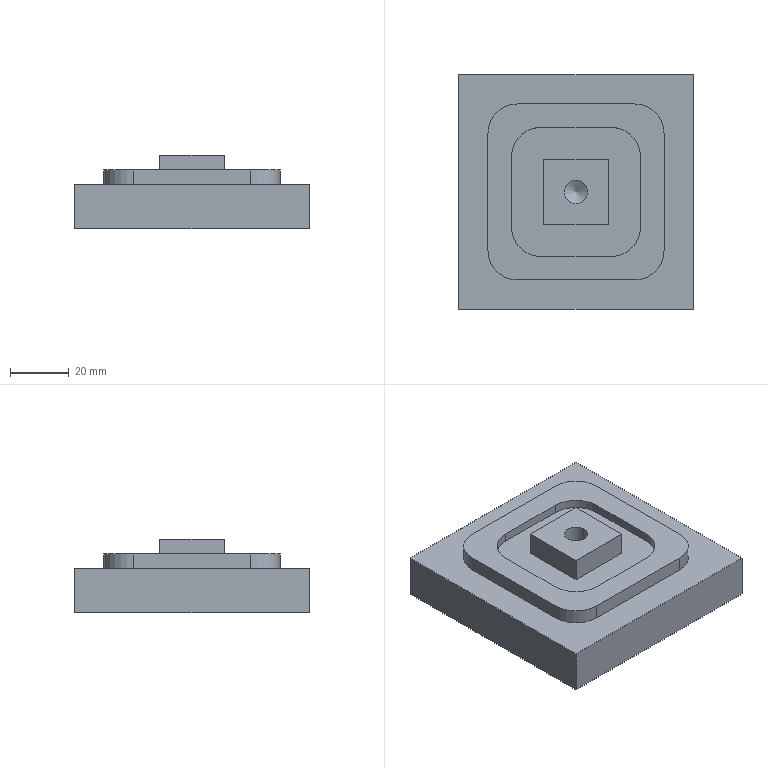Part | NX | 1 solid | 31 faces | box 80 x 80 x 25 mm | volume 111450 mm3 | plane 21 | cylinder 9 | cone 1 | commonest cylinder face diameters 20 x8 8 x1
STEP:
#1=CARTESIAN_POINT('',(-12.,-22.,17.));
#2=VERTEX_POINT('',#1);
#3=CARTESIAN_POINT('',(12.,-22.,17.));
#4=VERTEX_POINT('',#3);
#5=CARTESIAN_POINT('',(-22.,-22.,17.));
#6=DIRECTION('',(1.,0.,0.));
#7=VECTOR('',#6,1000.);
#8=LINE('',#5,#7);
#9=EDGE_CURVE('',#2,#4,#8,.T.);
#10=ORIENTED_EDGE('',*,*,#9,.T.);
#11=CARTESIAN_POINT('',(22.,-12.,17.));
#12=VERTEX_POINT('',#11);
#13=CARTESIAN_POINT('',(12.,-12.,17.));
#14=DIRECTION('',(0.,0.,1.));
#15=DIRECTION('',(1.,0.,0.));
#16=AXIS2_PLACEMENT_3D('',#13,#14,#15);
#17=CIRCLE('',#16,10.);
#18=EDGE_CURVE('',#4,#12,#17,.T.);
#19=ORIENTED_EDGE('',*,*,#18,.T.);
#20=CARTESIAN_POINT('',(22.,12.,17.));
#21=VERTEX_POINT('',#20);
#22=CARTESIAN_POINT('',(22.,-22.,17.));
#23=DIRECTION('',(0.,1.,0.));
#24=VECTOR('',#23,1000.);
#25=LINE('',#22,#24);
#26=EDGE_CURVE('',#12,#21,#25,.T.);
#27=ORIENTED_EDGE('',*,*,#26,.T.);
#28=CARTESIAN_POINT('',(12.,22.,17.));
#29=VERTEX_POINT('',#28);
#30=CARTESIAN_POINT('',(12.,12.,17.));
#31=DIRECTION('',(0.,0.,1.));
#32=DIRECTION('',(1.,0.,0.));
#33=AXIS2_PLACEMENT_3D('',#30,#31,#32);
#34=CIRCLE('',#33,10.);
#35=EDGE_CURVE('',#21,#29,#34,.T.);
#36=ORIENTED_EDGE('',*,*,#35,.T.);
#37=CARTESIAN_POINT('',(-12.,22.,17.));
#38=VERTEX_POINT('',#37);
#39=CARTESIAN_POINT('',(22.,22.,17.));
#40=DIRECTION('',(-1.,0.,0.));
#41=VECTOR('',#40,1000.);
#42=LINE('',#39,#41);
#43=EDGE_CURVE('',#29,#38,#42,.T.);
#44=ORIENTED_EDGE('',*,*,#43,.T.);
#45=CARTESIAN_POINT('',(-22.,12.,17.));
#46=VERTEX_POINT('',#45);
#47=CARTESIAN_POINT('',(-12.,12.,17.));
#48=DIRECTION('',(0.,0.,1.));
#49=DIRECTION('',(1.,0.,0.));
#50=AXIS2_PLACEMENT_3D('',#47,#48,#49);
#51=CIRCLE('',#50,10.);
#52=EDGE_CURVE('',#38,#46,#51,.T.);
#53=ORIENTED_EDGE('',*,*,#52,.T.);
#54=CARTESIAN_POINT('',(-22.,-12.,17.));
#55=VERTEX_POINT('',#54);
#56=CARTESIAN_POINT('',(-22.,22.,17.));
#57=DIRECTION('',(0.,-1.,0.));
#58=VECTOR('',#57,1000.);
#59=LINE('',#56,#58);
#60=EDGE_CURVE('',#46,#55,#59,.T.);
#61=ORIENTED_EDGE('',*,*,#60,.T.);
#62=CARTESIAN_POINT('',(-12.,-12.,17.));
#63=DIRECTION('',(0.,0.,1.));
#64=DIRECTION('',(1.,0.,0.));
#65=AXIS2_PLACEMENT_3D('',#62,#63,#64);
#66=CIRCLE('',#65,10.);
#67=EDGE_CURVE('',#55,#2,#66,.T.);
#68=ORIENTED_EDGE('',*,*,#67,.T.);
#69=EDGE_LOOP('',(#10,#19,#27,#36,#44,#53,#61,#68));
#70=FACE_BOUND('',#69,.T.);
#71=CARTESIAN_POINT('',(11.,11.,17.));
#72=VERTEX_POINT('',#71);
#73=CARTESIAN_POINT('',(11.,-11.,17.));
#74=VERTEX_POINT('',#73);
#75=CARTESIAN_POINT('',(11.,-22.,17.));
#76=DIRECTION('',(0.,-1.,0.));
#77=VECTOR('',#76,1000.);
#78=LINE('',#75,#77);
#79=EDGE_CURVE('',#72,#74,#78,.T.);
#80=ORIENTED_EDGE('',*,*,#79,.T.);
#81=CARTESIAN_POINT('',(-11.,-11.,17.));
#82=VERTEX_POINT('',#81);
#83=CARTESIAN_POINT('',(22.,-11.,17.));
#84=DIRECTION('',(-1.,0.,0.));
#85=VECTOR('',#84,1000.);
#86=LINE('',#83,#85);
#87=EDGE_CURVE('',#74,#82,#86,.T.);
#88=ORIENTED_EDGE('',*,*,#87,.T.);
#89=CARTESIAN_POINT('',(-11.,11.,17.));
#90=VERTEX_POINT('',#89);
#91=CARTESIAN_POINT('',(-11.,-22.,17.));
#92=DIRECTION('',(0.,1.,0.));
#93=VECTOR('',#92,1000.);
#94=LINE('',#91,#93);
#95=EDGE_CURVE('',#82,#90,#94,.T.);
#96=ORIENTED_EDGE('',*,*,#95,.T.);
#97=CARTESIAN_POINT('',(22.,11.,17.));
#98=DIRECTION('',(1.,0.,0.));
#99=VECTOR('',#98,1000.);
#100=LINE('',#97,#99);
#101=EDGE_CURVE('',#90,#72,#100,.T.);
#102=ORIENTED_EDGE('',*,*,#101,.T.);
#103=EDGE_LOOP('',(#80,#88,#96,#102));
#104=FACE_BOUND('',#103,.T.);
#105=CARTESIAN_POINT('',(22.,-22.,17.));
#106=DIRECTION('',(0.,0.,1.));
#107=DIRECTION('',(1.,0.,0.));
#108=AXIS2_PLACEMENT_3D('',#105,#106,#107);
#109=PLANE('',#108);
#110=ADVANCED_FACE('',(#70,#104),#109,.T.);
#111=CARTESIAN_POINT('',(30.,-20.,20.));
#112=VERTEX_POINT('',#111);
#113=CARTESIAN_POINT('',(30.,20.,20.));
#114=VERTEX_POINT('',#113);
#115=CARTESIAN_POINT('',(30.,-30.,20.));
#116=DIRECTION('',(0.,1.,0.));
#117=VECTOR('',#116,1000.);
#118=LINE('',#115,#117);
#119=EDGE_CURVE('',#112,#114,#118,.T.);
#120=ORIENTED_EDGE('',*,*,#119,.T.);
#121=CARTESIAN_POINT('',(20.,30.,20.));
#122=VERTEX_POINT('',#121);
#123=CARTESIAN_POINT('',(20.,20.,20.));
#124=DIRECTION('',(0.,0.,1.));
#125=DIRECTION('',(1.,0.,0.));
#126=AXIS2_PLACEMENT_3D('',#123,#124,#125);
#127=CIRCLE('',#126,10.);
#128=EDGE_CURVE('',#114,#122,#127,.T.);
#129=ORIENTED_EDGE('',*,*,#128,.T.);
#130=CARTESIAN_POINT('',(-20.,30.,20.));
#131=VERTEX_POINT('',#130);
#132=CARTESIAN_POINT('',(30.,30.,20.));
#133=DIRECTION('',(-1.,0.,0.));
#134=VECTOR('',#133,1000.);
#135=LINE('',#132,#134);
#136=EDGE_CURVE('',#122,#131,#135,.T.);
#137=ORIENTED_EDGE('',*,*,#136,.T.);
#138=CARTESIAN_POINT('',(-30.,20.,20.));
#139=VERTEX_POINT('',#138);
#140=CARTESIAN_POINT('',(-20.,20.,20.));
#141=DIRECTION('',(0.,0.,1.));
#142=DIRECTION('',(1.,0.,0.));
#143=AXIS2_PLACEMENT_3D('',#140,#141,#142);
#144=CIRCLE('',#143,10.);
#145=EDGE_CURVE('',#131,#139,#144,.T.);
#146=ORIENTED_EDGE('',*,*,#145,.T.);
#147=CARTESIAN_POINT('',(-30.,-20.,20.));
#148=VERTEX_POINT('',#147);
#149=CARTESIAN_POINT('',(-30.,30.,20.));
#150=DIRECTION('',(0.,-1.,0.));
#151=VECTOR('',#150,1000.);
#152=LINE('',#149,#151);
#153=EDGE_CURVE('',#139,#148,#152,.T.);
#154=ORIENTED_EDGE('',*,*,#153,.T.);
#155=CARTESIAN_POINT('',(-20.,-30.,20.));
#156=VERTEX_POINT('',#155);
#157=CARTESIAN_POINT('',(-20.,-20.,20.));
#158=DIRECTION('',(0.,0.,1.));
#159=DIRECTION('',(1.,0.,0.));
#160=AXIS2_PLACEMENT_3D('',#157,#158,#159);
#161=CIRCLE('',#160,10.);
#162=EDGE_CURVE('',#148,#156,#161,.T.);
#163=ORIENTED_EDGE('',*,*,#162,.T.);
#164=CARTESIAN_POINT('',(20.,-30.,20.));
#165=VERTEX_POINT('',#164);
#166=CARTESIAN_POINT('',(-30.,-30.,20.));
#167=DIRECTION('',(1.,0.,0.));
#168=VECTOR('',#167,1000.);
#169=LINE('',#166,#168);
#170=EDGE_CURVE('',#156,#165,#169,.T.);
#171=ORIENTED_EDGE('',*,*,#170,.T.);
#172=CARTESIAN_POINT('',(20.,-20.,20.));
#173=DIRECTION('',(0.,0.,1.));
#174=DIRECTION('',(1.,0.,0.));
#175=AXIS2_PLACEMENT_3D('',#172,#173,#174);
#176=CIRCLE('',#175,10.);
#177=EDGE_CURVE('',#165,#112,#176,.T.);
#178=ORIENTED_EDGE('',*,*,#177,.T.);
#179=EDGE_LOOP('',(#120,#129,#137,#146,#154,#163,#171,#178));
#180=FACE_BOUND('',#179,.T.);
#181=CARTESIAN_POINT('',(22.,-12.,20.));
#182=VERTEX_POINT('',#181);
#183=CARTESIAN_POINT('',(22.,12.,20.));
#184=VERTEX_POINT('',#183);
#185=CARTESIAN_POINT('',(22.,-22.,20.));
#186=DIRECTION('',(0.,1.,0.));
#187=VECTOR('',#186,1000.);
#188=LINE('',#185,#187);
#189=EDGE_CURVE('',#182,#184,#188,.T.);
#190=ORIENTED_EDGE('',*,*,#189,.F.);
#191=CARTESIAN_POINT('',(12.,-22.,20.));
#192=VERTEX_POINT('',#191);
#193=CARTESIAN_POINT('',(12.,-12.,20.));
#194=DIRECTION('',(0.,0.,1.));
#195=DIRECTION('',(1.,0.,0.));
#196=AXIS2_PLACEMENT_3D('',#193,#194,#195);
#197=CIRCLE('',#196,10.);
#198=EDGE_CURVE('',#182,#192,#197,.F.);
#199=ORIENTED_EDGE('',*,*,#198,.T.);
#200=CARTESIAN_POINT('',(-12.,-22.,20.));
#201=VERTEX_POINT('',#200);
#202=CARTESIAN_POINT('',(-22.,-22.,20.));
#203=DIRECTION('',(1.,0.,0.));
#204=VECTOR('',#203,1000.);
#205=LINE('',#202,#204);
#206=EDGE_CURVE('',#201,#192,#205,.T.);
#207=ORIENTED_EDGE('',*,*,#206,.F.);
#208=CARTESIAN_POINT('',(-22.,-12.,20.));
#209=VERTEX_POINT('',#208);
#210=CARTESIAN_POINT('',(-12.,-12.,20.));
#211=DIRECTION('',(0.,0.,1.));
#212=DIRECTION('',(1.,0.,0.));
#213=AXIS2_PLACEMENT_3D('',#210,#211,#212);
#214=CIRCLE('',#213,10.);
#215=EDGE_CURVE('',#201,#209,#214,.F.);
#216=ORIENTED_EDGE('',*,*,#215,.T.);
#217=CARTESIAN_POINT('',(-22.,12.,20.));
#218=VERTEX_POINT('',#217);
#219=CARTESIAN_POINT('',(-22.,22.,20.));
#220=DIRECTION('',(0.,-1.,0.));
#221=VECTOR('',#220,1000.);
#222=LINE('',#219,#221);
#223=EDGE_CURVE('',#218,#209,#222,.T.);
#224=ORIENTED_EDGE('',*,*,#223,.F.);
#225=CARTESIAN_POINT('',(-12.,22.,20.));
#226=VERTEX_POINT('',#225);
#227=CARTESIAN_POINT('',(-12.,12.,20.));
#228=DIRECTION('',(0.,0.,1.));
#229=DIRECTION('',(1.,0.,0.));
#230=AXIS2_PLACEMENT_3D('',#227,#228,#229);
#231=CIRCLE('',#230,10.);
#232=EDGE_CURVE('',#218,#226,#231,.F.);
#233=ORIENTED_EDGE('',*,*,#232,.T.);
#234=CARTESIAN_POINT('',(12.,22.,20.));
#235=VERTEX_POINT('',#234);
#236=CARTESIAN_POINT('',(22.,22.,20.));
#237=DIRECTION('',(-1.,0.,0.));
#238=VECTOR('',#237,1000.);
#239=LINE('',#236,#238);
#240=EDGE_CURVE('',#235,#226,#239,.T.);
#241=ORIENTED_EDGE('',*,*,#240,.F.);
#242=CARTESIAN_POINT('',(12.,12.,20.));
#243=DIRECTION('',(0.,0.,1.));
#244=DIRECTION('',(1.,0.,0.));
#245=AXIS2_PLACEMENT_3D('',#242,#243,#244);
#246=CIRCLE('',#245,10.);
#247=EDGE_CURVE('',#235,#184,#246,.F.);
#248=ORIENTED_EDGE('',*,*,#247,.T.);
#249=EDGE_LOOP('',(#190,#199,#207,#216,#224,#233,#241,#248));
#250=FACE_BOUND('',#249,.T.);
#251=CARTESIAN_POINT('',(30.,-30.,20.));
#252=DIRECTION('',(0.,0.,1.));
#253=DIRECTION('',(1.,0.,0.));
#254=AXIS2_PLACEMENT_3D('',#251,#252,#253);
#255=PLANE('',#254);
#256=ADVANCED_FACE('',(#180,#250),#255,.T.);
#257=CARTESIAN_POINT('',(-40.,-40.,15.));
#258=VERTEX_POINT('',#257);
#259=CARTESIAN_POINT('',(40.,-40.,15.));
#260=VERTEX_POINT('',#259);
#261=CARTESIAN_POINT('',(-40.,-40.,15.));
#262=DIRECTION('',(1.,0.,0.));
#263=VECTOR('',#262,1000.);
#264=LINE('',#261,#263);
#265=EDGE_CURVE('',#258,#260,#264,.T.);
#266=ORIENTED_EDGE('',*,*,#265,.T.);
#267=CARTESIAN_POINT('',(40.,40.,15.));
#268=VERTEX_POINT('',#267);
#269=CARTESIAN_POINT('',(40.,-40.,15.));
#270=DIRECTION('',(0.,1.,0.));
#271=VECTOR('',#270,1000.);
#272=LINE('',#269,#271);
#273=EDGE_CURVE('',#260,#268,#272,.T.);
#274=ORIENTED_EDGE('',*,*,#273,.T.);
#275=CARTESIAN_POINT('',(-40.,40.,15.));
#276=VERTEX_POINT('',#275);
#277=CARTESIAN_POINT('',(40.,40.,15.));
#278=DIRECTION('',(-1.,0.,0.));
#279=VECTOR('',#278,1000.);
#280=LINE('',#277,#279);
#281=EDGE_CURVE('',#268,#276,#280,.T.);
#282=ORIENTED_EDGE('',*,*,#281,.T.);
#283=CARTESIAN_POINT('',(-40.,40.,15.));
#284=DIRECTION('',(0.,-1.,0.));
#285=VECTOR('',#284,1000.);
#286=LINE('',#283,#285);
#287=EDGE_CURVE('',#276,#258,#286,.T.);
#288=ORIENTED_EDGE('',*,*,#287,.T.);
#289=EDGE_LOOP('',(#266,#274,#282,#288));
#290=FACE_BOUND('',#289,.T.);
#291=CARTESIAN_POINT('',(-20.,30.,15.));
#292=VERTEX_POINT('',#291);
#293=CARTESIAN_POINT('',(20.,30.,15.));
#294=VERTEX_POINT('',#293);
#295=CARTESIAN_POINT('',(40.,30.,15.));
#296=DIRECTION('',(1.,0.,0.));
#297=VECTOR('',#296,1000.);
#298=LINE('',#295,#297);
#299=EDGE_CURVE('',#292,#294,#298,.T.);
#300=ORIENTED_EDGE('',*,*,#299,.T.);
#301=CARTESIAN_POINT('',(30.,20.,15.));
#302=VERTEX_POINT('',#301);
#303=CARTESIAN_POINT('',(20.,20.,15.));
#304=DIRECTION('',(0.,0.,1.));
#305=DIRECTION('',(1.,0.,0.));
#306=AXIS2_PLACEMENT_3D('',#303,#304,#305);
#307=CIRCLE('',#306,10.);
#308=EDGE_CURVE('',#294,#302,#307,.F.);
#309=ORIENTED_EDGE('',*,*,#308,.T.);
#310=CARTESIAN_POINT('',(30.,-20.,15.));
#311=VERTEX_POINT('',#310);
#312=CARTESIAN_POINT('',(30.,-40.,15.));
#313=DIRECTION('',(0.,-1.,0.));
#314=VECTOR('',#313,1000.);
#315=LINE('',#312,#314);
#316=EDGE_CURVE('',#302,#311,#315,.T.);
#317=ORIENTED_EDGE('',*,*,#316,.T.);
#318=CARTESIAN_POINT('',(20.,-30.,15.));
#319=VERTEX_POINT('',#318);
#320=CARTESIAN_POINT('',(20.,-20.,15.));
#321=DIRECTION('',(0.,0.,1.));
#322=DIRECTION('',(1.,0.,0.));
#323=AXIS2_PLACEMENT_3D('',#320,#321,#322);
#324=CIRCLE('',#323,10.);
#325=EDGE_CURVE('',#311,#319,#324,.F.);
#326=ORIENTED_EDGE('',*,*,#325,.T.);
#327=CARTESIAN_POINT('',(-20.,-30.,15.));
#328=VERTEX_POINT('',#327);
#329=CARTESIAN_POINT('',(40.,-30.,15.));
#330=DIRECTION('',(-1.,0.,0.));
#331=VECTOR('',#330,1000.);
#332=LINE('',#329,#331);
#333=EDGE_CURVE('',#319,#328,#332,.T.);
#334=ORIENTED_EDGE('',*,*,#333,.T.);
#335=CARTESIAN_POINT('',(-30.,-20.,15.));
#336=VERTEX_POINT('',#335);
#337=CARTESIAN_POINT('',(-20.,-20.,15.));
#338=DIRECTION('',(0.,0.,1.));
#339=DIRECTION('',(1.,0.,0.));
#340=AXIS2_PLACEMENT_3D('',#337,#338,#339);
#341=CIRCLE('',#340,10.);
#342=EDGE_CURVE('',#328,#336,#341,.F.);
#343=ORIENTED_EDGE('',*,*,#342,.T.);
#344=CARTESIAN_POINT('',(-30.,20.,15.));
#345=VERTEX_POINT('',#344);
#346=CARTESIAN_POINT('',(-30.,-40.,15.));
#347=DIRECTION('',(0.,1.,0.));
#348=VECTOR('',#347,1000.);
#349=LINE('',#346,#348);
#350=EDGE_CURVE('',#336,#345,#349,.T.);
#351=ORIENTED_EDGE('',*,*,#350,.T.);
#352=CARTESIAN_POINT('',(-20.,20.,15.));
#353=DIRECTION('',(0.,0.,1.));
#354=DIRECTION('',(1.,0.,0.));
#355=AXIS2_PLACEMENT_3D('',#352,#353,#354);
#356=CIRCLE('',#355,10.);
#357=EDGE_CURVE('',#345,#292,#356,.F.);
#358=ORIENTED_EDGE('',*,*,#357,.T.);
#359=EDGE_LOOP('',(#300,#309,#317,#326,#334,#343,#351,#358));
#360=FACE_BOUND('',#359,.T.);
#361=CARTESIAN_POINT('',(40.,-40.,15.));
#362=DIRECTION('',(0.,0.,1.));
#363=DIRECTION('',(1.,0.,0.));
#364=AXIS2_PLACEMENT_3D('',#361,#362,#363);
#365=PLANE('',#364);
#366=ADVANCED_FACE('',(#290,#360),#365,.T.);
#367=CARTESIAN_POINT('',(-40.,-40.,0.));
#368=VERTEX_POINT('',#367);
#369=CARTESIAN_POINT('',(40.,-40.,0.));
#370=VERTEX_POINT('',#369);
#371=CARTESIAN_POINT('',(-40.,-40.,0.));
#372=DIRECTION('',(1.,0.,0.));
#373=VECTOR('',#372,1000.);
#374=LINE('',#371,#373);
#375=EDGE_CURVE('',#368,#370,#374,.T.);
#376=ORIENTED_EDGE('',*,*,#375,.T.);
#377=CARTESIAN_POINT('',(40.,-40.,15.));
#378=DIRECTION('',(0.,0.,-1.));
#379=VECTOR('',#378,1000.);
#380=LINE('',#377,#379);
#381=EDGE_CURVE('',#260,#370,#380,.T.);
#382=ORIENTED_EDGE('',*,*,#381,.F.);
#383=ORIENTED_EDGE('',*,*,#265,.F.);
#384=CARTESIAN_POINT('',(-40.,-40.,15.));
#385=DIRECTION('',(0.,0.,-1.));
#386=VECTOR('',#385,1000.);
#387=LINE('',#384,#386);
#388=EDGE_CURVE('',#258,#368,#387,.T.);
#389=ORIENTED_EDGE('',*,*,#388,.T.);
#390=EDGE_LOOP('',(#376,#382,#383,#389));
#391=FACE_BOUND('',#390,.T.);
#392=CARTESIAN_POINT('',(-40.,-40.,15.));
#393=DIRECTION('',(0.,1.,0.));
#394=DIRECTION('',(0.,0.,1.));
#395=AXIS2_PLACEMENT_3D('',#392,#393,#394);
#396=PLANE('',#395);
#397=ADVANCED_FACE('',(#391),#396,.F.);
#398=CARTESIAN_POINT('',(40.,40.,0.));
#399=VERTEX_POINT('',#398);
#400=CARTESIAN_POINT('',(40.,-40.,0.));
#401=DIRECTION('',(0.,1.,0.));
#402=VECTOR('',#401,1000.);
#403=LINE('',#400,#402);
#404=EDGE_CURVE('',#370,#399,#403,.T.);
#405=ORIENTED_EDGE('',*,*,#404,.T.);
#406=CARTESIAN_POINT('',(40.,40.,15.));
#407=DIRECTION('',(0.,0.,-1.));
#408=VECTOR('',#407,1000.);
#409=LINE('',#406,#408);
#410=EDGE_CURVE('',#268,#399,#409,.T.);
#411=ORIENTED_EDGE('',*,*,#410,.F.);
#412=ORIENTED_EDGE('',*,*,#273,.F.);
#413=ORIENTED_EDGE('',*,*,#381,.T.);
#414=EDGE_LOOP('',(#405,#411,#412,#413));
#415=FACE_BOUND('',#414,.T.);
#416=CARTESIAN_POINT('',(40.,-40.,15.));
#417=DIRECTION('',(-1.,0.,0.));
#418=DIRECTION('',(0.,-1.,0.));
#419=AXIS2_PLACEMENT_3D('',#416,#417,#418);
#420=PLANE('',#419);
#421=ADVANCED_FACE('',(#415),#420,.F.);
#422=CARTESIAN_POINT('',(-40.,40.,0.));
#423=VERTEX_POINT('',#422);
#424=CARTESIAN_POINT('',(40.,40.,0.));
#425=DIRECTION('',(-1.,0.,0.));
#426=VECTOR('',#425,1000.);
#427=LINE('',#424,#426);
#428=EDGE_CURVE('',#399,#423,#427,.T.);
#429=ORIENTED_EDGE('',*,*,#428,.T.);
#430=CARTESIAN_POINT('',(-40.,40.,15.));
#431=DIRECTION('',(0.,0.,-1.));
#432=VECTOR('',#431,1000.);
#433=LINE('',#430,#432);
#434=EDGE_CURVE('',#276,#423,#433,.T.);
#435=ORIENTED_EDGE('',*,*,#434,.F.);
#436=ORIENTED_EDGE('',*,*,#281,.F.);
#437=ORIENTED_EDGE('',*,*,#410,.T.);
#438=EDGE_LOOP('',(#429,#435,#436,#437));
#439=FACE_BOUND('',#438,.T.);
#440=CARTESIAN_POINT('',(40.,40.,15.));
#441=DIRECTION('',(0.,-1.,0.));
#442=DIRECTION('',(1.,0.,0.));
#443=AXIS2_PLACEMENT_3D('',#440,#441,#442);
#444=PLANE('',#443);
#445=ADVANCED_FACE('',(#439),#444,.F.);
#446=CARTESIAN_POINT('',(-40.,40.,0.));
#447=DIRECTION('',(0.,-1.,0.));
#448=VECTOR('',#447,1000.);
#449=LINE('',#446,#448);
#450=EDGE_CURVE('',#423,#368,#449,.T.);
#451=ORIENTED_EDGE('',*,*,#450,.T.);
#452=ORIENTED_EDGE('',*,*,#388,.F.);
#453=ORIENTED_EDGE('',*,*,#287,.F.);
#454=ORIENTED_EDGE('',*,*,#434,.T.);
#455=EDGE_LOOP('',(#451,#452,#453,#454));
#456=FACE_BOUND('',#455,.T.);
#457=CARTESIAN_POINT('',(-40.,40.,15.));
#458=DIRECTION('',(1.,0.,0.));
#459=DIRECTION('',(0.,1.,0.));
#460=AXIS2_PLACEMENT_3D('',#457,#458,#459);
#461=PLANE('',#460);
#462=ADVANCED_FACE('',(#456),#461,.F.);
#463=ORIENTED_EDGE('',*,*,#375,.F.);
#464=ORIENTED_EDGE('',*,*,#450,.F.);
#465=ORIENTED_EDGE('',*,*,#428,.F.);
#466=ORIENTED_EDGE('',*,*,#404,.F.);
#467=EDGE_LOOP('',(#463,#464,#465,#466));
#468=FACE_BOUND('',#467,.T.);
#469=CARTESIAN_POINT('',(40.,-40.,0.));
#470=DIRECTION('',(0.,0.,1.));
#471=DIRECTION('',(1.,0.,0.));
#472=AXIS2_PLACEMENT_3D('',#469,#470,#471);
#473=PLANE('',#472);
#474=ADVANCED_FACE('',(#468),#473,.F.);
#475=ORIENTED_EDGE('',*,*,#170,.F.);
#476=CARTESIAN_POINT('',(-20.,-30.,20.));
#477=DIRECTION('',(0.,0.,-1.));
#478=VECTOR('',#477,1000.);
#479=LINE('',#476,#478);
#480=EDGE_CURVE('',#156,#328,#479,.T.);
#481=ORIENTED_EDGE('',*,*,#480,.T.);
#482=ORIENTED_EDGE('',*,*,#333,.F.);
#483=CARTESIAN_POINT('',(20.,-30.,20.));
#484=DIRECTION('',(0.,0.,-1.));
#485=VECTOR('',#484,1000.);
#486=LINE('',#483,#485);
#487=EDGE_CURVE('',#319,#165,#486,.F.);
#488=ORIENTED_EDGE('',*,*,#487,.T.);
#489=EDGE_LOOP('',(#475,#481,#482,#488));
#490=FACE_BOUND('',#489,.T.);
#491=CARTESIAN_POINT('',(-30.,-30.,20.));
#492=DIRECTION('',(0.,1.,0.));
#493=DIRECTION('',(0.,0.,1.));
#494=AXIS2_PLACEMENT_3D('',#491,#492,#493);
#495=PLANE('',#494);
#496=ADVANCED_FACE('',(#490),#495,.F.);
#497=ORIENTED_EDGE('',*,*,#316,.F.);
#498=CARTESIAN_POINT('',(30.,20.,20.));
#499=DIRECTION('',(0.,0.,-1.));
#500=VECTOR('',#499,1000.);
#501=LINE('',#498,#500);
#502=EDGE_CURVE('',#302,#114,#501,.F.);
#503=ORIENTED_EDGE('',*,*,#502,.T.);
#504=ORIENTED_EDGE('',*,*,#119,.F.);
#505=CARTESIAN_POINT('',(30.,-20.,20.));
#506=DIRECTION('',(0.,0.,-1.));
#507=VECTOR('',#506,1000.);
#508=LINE('',#505,#507);
#509=EDGE_CURVE('',#112,#311,#508,.T.);
#510=ORIENTED_EDGE('',*,*,#509,.T.);
#511=EDGE_LOOP('',(#497,#503,#504,#510));
#512=FACE_BOUND('',#511,.T.);
#513=CARTESIAN_POINT('',(30.,-30.,20.));
#514=DIRECTION('',(-1.,0.,0.));
#515=DIRECTION('',(0.,-1.,0.));
#516=AXIS2_PLACEMENT_3D('',#513,#514,#515);
#517=PLANE('',#516);
#518=ADVANCED_FACE('',(#512),#517,.F.);
#519=ORIENTED_EDGE('',*,*,#136,.F.);
#520=CARTESIAN_POINT('',(20.,30.,20.));
#521=DIRECTION('',(0.,0.,-1.));
#522=VECTOR('',#521,1000.);
#523=LINE('',#520,#522);
#524=EDGE_CURVE('',#122,#294,#523,.T.);
#525=ORIENTED_EDGE('',*,*,#524,.T.);
#526=ORIENTED_EDGE('',*,*,#299,.F.);
#527=CARTESIAN_POINT('',(-20.,30.,20.));
#528=DIRECTION('',(0.,0.,-1.));
#529=VECTOR('',#528,1000.);
#530=LINE('',#527,#529);
#531=EDGE_CURVE('',#292,#131,#530,.F.);
#532=ORIENTED_EDGE('',*,*,#531,.T.);
#533=EDGE_LOOP('',(#519,#525,#526,#532));
#534=FACE_BOUND('',#533,.T.);
#535=CARTESIAN_POINT('',(30.,30.,20.));
#536=DIRECTION('',(0.,-1.,0.));
#537=DIRECTION('',(1.,0.,0.));
#538=AXIS2_PLACEMENT_3D('',#535,#536,#537);
#539=PLANE('',#538);
#540=ADVANCED_FACE('',(#534),#539,.F.);
#541=ORIENTED_EDGE('',*,*,#153,.F.);
#542=CARTESIAN_POINT('',(-30.,20.,20.));
#543=DIRECTION('',(0.,0.,-1.));
#544=VECTOR('',#543,1000.);
#545=LINE('',#542,#544);
#546=EDGE_CURVE('',#139,#345,#545,.T.);
#547=ORIENTED_EDGE('',*,*,#546,.T.);
#548=ORIENTED_EDGE('',*,*,#350,.F.);
#549=CARTESIAN_POINT('',(-30.,-20.,20.));
#550=DIRECTION('',(0.,0.,-1.));
#551=VECTOR('',#550,1000.);
#552=LINE('',#549,#551);
#553=EDGE_CURVE('',#336,#148,#552,.F.);
#554=ORIENTED_EDGE('',*,*,#553,.T.);
#555=EDGE_LOOP('',(#541,#547,#548,#554));
#556=FACE_BOUND('',#555,.T.);
#557=CARTESIAN_POINT('',(-30.,30.,20.));
#558=DIRECTION('',(1.,0.,0.));
#559=DIRECTION('',(0.,1.,0.));
#560=AXIS2_PLACEMENT_3D('',#557,#558,#559);
#561=PLANE('',#560);
#562=ADVANCED_FACE('',(#556),#561,.F.);
#563=ORIENTED_EDGE('',*,*,#206,.T.);
#564=CARTESIAN_POINT('',(12.,-22.,17.));
#565=DIRECTION('',(0.,0.,-1.));
#566=VECTOR('',#565,1000.);
#567=LINE('',#564,#566);
#568=EDGE_CURVE('',#192,#4,#567,.T.);
#569=ORIENTED_EDGE('',*,*,#568,.T.);
#570=ORIENTED_EDGE('',*,*,#9,.F.);
#571=CARTESIAN_POINT('',(-12.,-22.,20.));
#572=DIRECTION('',(0.,0.,-1.));
#573=VECTOR('',#572,1000.);
#574=LINE('',#571,#573);
#575=EDGE_CURVE('',#2,#201,#574,.F.);
#576=ORIENTED_EDGE('',*,*,#575,.T.);
#577=EDGE_LOOP('',(#563,#569,#570,#576));
#578=FACE_BOUND('',#577,.T.);
#579=CARTESIAN_POINT('',(-22.,-22.,20.));
#580=DIRECTION('',(0.,1.,0.));
#581=DIRECTION('',(0.,0.,1.));
#582=AXIS2_PLACEMENT_3D('',#579,#580,#581);
#583=PLANE('',#582);
#584=ADVANCED_FACE('',(#578),#583,.T.);
#585=ORIENTED_EDGE('',*,*,#26,.F.);
#586=CARTESIAN_POINT('',(22.,-12.,20.));
#587=DIRECTION('',(0.,0.,-1.));
#588=VECTOR('',#587,1000.);
#589=LINE('',#586,#588);
#590=EDGE_CURVE('',#12,#182,#589,.F.);
#591=ORIENTED_EDGE('',*,*,#590,.T.);
#592=ORIENTED_EDGE('',*,*,#189,.T.);
#593=CARTESIAN_POINT('',(22.,12.,17.));
#594=DIRECTION('',(0.,0.,-1.));
#595=VECTOR('',#594,1000.);
#596=LINE('',#593,#595);
#597=EDGE_CURVE('',#184,#21,#596,.T.);
#598=ORIENTED_EDGE('',*,*,#597,.T.);
#599=EDGE_LOOP('',(#585,#591,#592,#598));
#600=FACE_BOUND('',#599,.T.);
#601=CARTESIAN_POINT('',(22.,-22.,20.));
#602=DIRECTION('',(-1.,0.,0.));
#603=DIRECTION('',(0.,-1.,0.));
#604=AXIS2_PLACEMENT_3D('',#601,#602,#603);
#605=PLANE('',#604);
#606=ADVANCED_FACE('',(#600),#605,.T.);
#607=ORIENTED_EDGE('',*,*,#43,.F.);
#608=CARTESIAN_POINT('',(12.,22.,20.));
#609=DIRECTION('',(0.,0.,-1.));
#610=VECTOR('',#609,1000.);
#611=LINE('',#608,#610);
#612=EDGE_CURVE('',#29,#235,#611,.F.);
#613=ORIENTED_EDGE('',*,*,#612,.T.);
#614=ORIENTED_EDGE('',*,*,#240,.T.);
#615=CARTESIAN_POINT('',(-12.,22.,17.));
#616=DIRECTION('',(0.,0.,-1.));
#617=VECTOR('',#616,1000.);
#618=LINE('',#615,#617);
#619=EDGE_CURVE('',#226,#38,#618,.T.);
#620=ORIENTED_EDGE('',*,*,#619,.T.);
#621=EDGE_LOOP('',(#607,#613,#614,#620));
#622=FACE_BOUND('',#621,.T.);
#623=CARTESIAN_POINT('',(22.,22.,20.));
#624=DIRECTION('',(0.,-1.,0.));
#625=DIRECTION('',(1.,0.,0.));
#626=AXIS2_PLACEMENT_3D('',#623,#624,#625);
#627=PLANE('',#626);
#628=ADVANCED_FACE('',(#622),#627,.T.);
#629=ORIENTED_EDGE('',*,*,#223,.T.);
#630=CARTESIAN_POINT('',(-22.,-12.,17.));
#631=DIRECTION('',(0.,0.,-1.));
#632=VECTOR('',#631,1000.);
#633=LINE('',#630,#632);
#634=EDGE_CURVE('',#209,#55,#633,.T.);
#635=ORIENTED_EDGE('',*,*,#634,.T.);
#636=ORIENTED_EDGE('',*,*,#60,.F.);
#637=CARTESIAN_POINT('',(-22.,12.,20.));
#638=DIRECTION('',(0.,0.,-1.));
#639=VECTOR('',#638,1000.);
#640=LINE('',#637,#639);
#641=EDGE_CURVE('',#46,#218,#640,.F.);
#642=ORIENTED_EDGE('',*,*,#641,.T.);
#643=EDGE_LOOP('',(#629,#635,#636,#642));
#644=FACE_BOUND('',#643,.T.);
#645=CARTESIAN_POINT('',(-22.,22.,20.));
#646=DIRECTION('',(1.,0.,0.));
#647=DIRECTION('',(0.,1.,0.));
#648=AXIS2_PLACEMENT_3D('',#645,#646,#647);
#649=PLANE('',#648);
#650=ADVANCED_FACE('',(#644),#649,.T.);
#651=ORIENTED_EDGE('',*,*,#87,.F.);
#652=CARTESIAN_POINT('',(11.,-11.,25.));
#653=VERTEX_POINT('',#652);
#654=CARTESIAN_POINT('',(11.,-11.,25.));
#655=DIRECTION('',(0.,0.,-1.));
#656=VECTOR('',#655,1000.);
#657=LINE('',#654,#656);
#658=EDGE_CURVE('',#653,#74,#657,.T.);
#659=ORIENTED_EDGE('',*,*,#658,.F.);
#660=CARTESIAN_POINT('',(-11.,-11.,25.));
#661=VERTEX_POINT('',#660);
#662=CARTESIAN_POINT('',(-11.,-11.,25.));
#663=DIRECTION('',(1.,0.,0.));
#664=VECTOR('',#663,1000.);
#665=LINE('',#662,#664);
#666=EDGE_CURVE('',#661,#653,#665,.T.);
#667=ORIENTED_EDGE('',*,*,#666,.F.);
#668=CARTESIAN_POINT('',(-11.,-11.,25.));
#669=DIRECTION('',(0.,0.,-1.));
#670=VECTOR('',#669,1000.);
#671=LINE('',#668,#670);
#672=EDGE_CURVE('',#661,#82,#671,.T.);
#673=ORIENTED_EDGE('',*,*,#672,.T.);
#674=EDGE_LOOP('',(#651,#659,#667,#673));
#675=FACE_BOUND('',#674,.T.);
#676=CARTESIAN_POINT('',(-11.,-11.,25.));
#677=DIRECTION('',(0.,1.,0.));
#678=DIRECTION('',(0.,0.,1.));
#679=AXIS2_PLACEMENT_3D('',#676,#677,#678);
#680=PLANE('',#679);
#681=ADVANCED_FACE('',(#675),#680,.F.);
#682=ORIENTED_EDGE('',*,*,#79,.F.);
#683=CARTESIAN_POINT('',(11.,11.,25.));
#684=VERTEX_POINT('',#683);
#685=CARTESIAN_POINT('',(11.,11.,25.));
#686=DIRECTION('',(0.,0.,-1.));
#687=VECTOR('',#686,1000.);
#688=LINE('',#685,#687);
#689=EDGE_CURVE('',#684,#72,#688,.T.);
#690=ORIENTED_EDGE('',*,*,#689,.F.);
#691=CARTESIAN_POINT('',(11.,-11.,25.));
#692=DIRECTION('',(0.,1.,0.));
#693=VECTOR('',#692,1000.);
#694=LINE('',#691,#693);
#695=EDGE_CURVE('',#653,#684,#694,.T.);
#696=ORIENTED_EDGE('',*,*,#695,.F.);
#697=ORIENTED_EDGE('',*,*,#658,.T.);
#698=EDGE_LOOP('',(#682,#690,#696,#697));
#699=FACE_BOUND('',#698,.T.);
#700=CARTESIAN_POINT('',(11.,-11.,25.));
#701=DIRECTION('',(-1.,0.,0.));
#702=DIRECTION('',(0.,-1.,0.));
#703=AXIS2_PLACEMENT_3D('',#700,#701,#702);
#704=PLANE('',#703);
#705=ADVANCED_FACE('',(#699),#704,.F.);
#706=ORIENTED_EDGE('',*,*,#101,.F.);
#707=CARTESIAN_POINT('',(-11.,11.,25.));
#708=VERTEX_POINT('',#707);
#709=CARTESIAN_POINT('',(-11.,11.,25.));
#710=DIRECTION('',(0.,0.,-1.));
#711=VECTOR('',#710,1000.);
#712=LINE('',#709,#711);
#713=EDGE_CURVE('',#708,#90,#712,.T.);
#714=ORIENTED_EDGE('',*,*,#713,.F.);
#715=CARTESIAN_POINT('',(11.,11.,25.));
#716=DIRECTION('',(-1.,0.,0.));
#717=VECTOR('',#716,1000.);
#718=LINE('',#715,#717);
#719=EDGE_CURVE('',#684,#708,#718,.T.);
#720=ORIENTED_EDGE('',*,*,#719,.F.);
#721=ORIENTED_EDGE('',*,*,#689,.T.);
#722=EDGE_LOOP('',(#706,#714,#720,#721));
#723=FACE_BOUND('',#722,.T.);
#724=CARTESIAN_POINT('',(11.,11.,25.));
#725=DIRECTION('',(0.,-1.,0.));
#726=DIRECTION('',(1.,0.,0.));
#727=AXIS2_PLACEMENT_3D('',#724,#725,#726);
#728=PLANE('',#727);
#729=ADVANCED_FACE('',(#723),#728,.F.);
#730=ORIENTED_EDGE('',*,*,#95,.F.);
#731=ORIENTED_EDGE('',*,*,#672,.F.);
#732=CARTESIAN_POINT('',(-11.,11.,25.));
#733=DIRECTION('',(0.,-1.,0.));
#734=VECTOR('',#733,1000.);
#735=LINE('',#732,#734);
#736=EDGE_CURVE('',#708,#661,#735,.T.);
#737=ORIENTED_EDGE('',*,*,#736,.F.);
#738=ORIENTED_EDGE('',*,*,#713,.T.);
#739=EDGE_LOOP('',(#730,#731,#737,#738));
#740=FACE_BOUND('',#739,.T.);
#741=CARTESIAN_POINT('',(-11.,11.,25.));
#742=DIRECTION('',(1.,0.,0.));
#743=DIRECTION('',(0.,1.,0.));
#744=AXIS2_PLACEMENT_3D('',#741,#742,#743);
#745=PLANE('',#744);
#746=ADVANCED_FACE('',(#740),#745,.F.);
#747=CARTESIAN_POINT('',(-4.,0.,25.));
#748=VERTEX_POINT('',#747);
#749=CARTESIAN_POINT('',(0.,0.,25.));
#750=DIRECTION('',(0.,0.,-1.));
#751=DIRECTION('',(-1.,0.,0.));
#752=AXIS2_PLACEMENT_3D('',#749,#750,#751);
#753=CIRCLE('',#752,4.);
#754=EDGE_CURVE('',#748,#748,#753,.T.);
#755=ORIENTED_EDGE('',*,*,#754,.T.);
#756=EDGE_LOOP('',(#755));
#757=FACE_BOUND('',#756,.T.);
#758=ORIENTED_EDGE('',*,*,#666,.T.);
#759=ORIENTED_EDGE('',*,*,#695,.T.);
#760=ORIENTED_EDGE('',*,*,#719,.T.);
#761=ORIENTED_EDGE('',*,*,#736,.T.);
#762=EDGE_LOOP('',(#758,#759,#760,#761));
#763=FACE_BOUND('',#762,.T.);
#764=CARTESIAN_POINT('',(11.,-11.,25.));
#765=DIRECTION('',(0.,0.,1.));
#766=DIRECTION('',(1.,0.,0.));
#767=AXIS2_PLACEMENT_3D('',#764,#765,#766);
#768=PLANE('',#767);
#769=ADVANCED_FACE('',(#757,#763),#768,.T.);
#770=ORIENTED_EDGE('',*,*,#128,.F.);
#771=ORIENTED_EDGE('',*,*,#502,.F.);
#772=ORIENTED_EDGE('',*,*,#308,.F.);
#773=ORIENTED_EDGE('',*,*,#524,.F.);
#774=EDGE_LOOP('',(#770,#771,#772,#773));
#775=FACE_BOUND('',#774,.T.);
#776=CARTESIAN_POINT('',(20.,20.,20.));
#777=DIRECTION('',(0.,0.,-1.));
#778=DIRECTION('',(-1.,0.,0.));
#779=AXIS2_PLACEMENT_3D('',#776,#777,#778);
#780=CYLINDRICAL_SURFACE('',#779,10.);
#781=ADVANCED_FACE('',(#775),#780,.T.);
#782=ORIENTED_EDGE('',*,*,#145,.F.);
#783=ORIENTED_EDGE('',*,*,#531,.F.);
#784=ORIENTED_EDGE('',*,*,#357,.F.);
#785=ORIENTED_EDGE('',*,*,#546,.F.);
#786=EDGE_LOOP('',(#782,#783,#784,#785));
#787=FACE_BOUND('',#786,.T.);
#788=CARTESIAN_POINT('',(-20.,20.,20.));
#789=DIRECTION('',(0.,0.,-1.));
#790=DIRECTION('',(-1.,0.,0.));
#791=AXIS2_PLACEMENT_3D('',#788,#789,#790);
#792=CYLINDRICAL_SURFACE('',#791,10.);
#793=ADVANCED_FACE('',(#787),#792,.T.);
#794=ORIENTED_EDGE('',*,*,#198,.F.);
#795=ORIENTED_EDGE('',*,*,#590,.F.);
#796=ORIENTED_EDGE('',*,*,#18,.F.);
#797=ORIENTED_EDGE('',*,*,#568,.F.);
#798=EDGE_LOOP('',(#794,#795,#796,#797));
#799=FACE_BOUND('',#798,.T.);
#800=CARTESIAN_POINT('',(12.,-12.,20.));
#801=DIRECTION('',(0.,0.,1.));
#802=DIRECTION('',(1.,0.,0.));
#803=AXIS2_PLACEMENT_3D('',#800,#801,#802);
#804=CYLINDRICAL_SURFACE('',#803,10.);
#805=ADVANCED_FACE('',(#799),#804,.F.);
#806=ORIENTED_EDGE('',*,*,#215,.F.);
#807=ORIENTED_EDGE('',*,*,#575,.F.);
#808=ORIENTED_EDGE('',*,*,#67,.F.);
#809=ORIENTED_EDGE('',*,*,#634,.F.);
#810=EDGE_LOOP('',(#806,#807,#808,#809));
#811=FACE_BOUND('',#810,.T.);
#812=CARTESIAN_POINT('',(-12.,-12.,20.));
#813=DIRECTION('',(0.,0.,1.));
#814=DIRECTION('',(1.,0.,0.));
#815=AXIS2_PLACEMENT_3D('',#812,#813,#814);
#816=CYLINDRICAL_SURFACE('',#815,10.);
#817=ADVANCED_FACE('',(#811),#816,.F.);
#818=ORIENTED_EDGE('',*,*,#247,.F.);
#819=ORIENTED_EDGE('',*,*,#612,.F.);
#820=ORIENTED_EDGE('',*,*,#35,.F.);
#821=ORIENTED_EDGE('',*,*,#597,.F.);
#822=EDGE_LOOP('',(#818,#819,#820,#821));
#823=FACE_BOUND('',#822,.T.);
#824=CARTESIAN_POINT('',(12.,12.,20.));
#825=DIRECTION('',(0.,0.,1.));
#826=DIRECTION('',(1.,0.,0.));
#827=AXIS2_PLACEMENT_3D('',#824,#825,#826);
#828=CYLINDRICAL_SURFACE('',#827,10.);
#829=ADVANCED_FACE('',(#823),#828,.F.);
#830=ORIENTED_EDGE('',*,*,#232,.F.);
#831=ORIENTED_EDGE('',*,*,#641,.F.);
#832=ORIENTED_EDGE('',*,*,#52,.F.);
#833=ORIENTED_EDGE('',*,*,#619,.F.);
#834=EDGE_LOOP('',(#830,#831,#832,#833));
#835=FACE_BOUND('',#834,.T.);
#836=CARTESIAN_POINT('',(-12.,12.,20.));
#837=DIRECTION('',(0.,0.,1.));
#838=DIRECTION('',(1.,0.,0.));
#839=AXIS2_PLACEMENT_3D('',#836,#837,#838);
#840=CYLINDRICAL_SURFACE('',#839,10.);
#841=ADVANCED_FACE('',(#835),#840,.F.);
#842=ORIENTED_EDGE('',*,*,#162,.F.);
#843=ORIENTED_EDGE('',*,*,#553,.F.);
#844=ORIENTED_EDGE('',*,*,#342,.F.);
#845=ORIENTED_EDGE('',*,*,#480,.F.);
#846=EDGE_LOOP('',(#842,#843,#844,#845));
#847=FACE_BOUND('',#846,.T.);
#848=CARTESIAN_POINT('',(-20.,-20.,20.));
#849=DIRECTION('',(0.,0.,-1.));
#850=DIRECTION('',(-1.,0.,0.));
#851=AXIS2_PLACEMENT_3D('',#848,#849,#850);
#852=CYLINDRICAL_SURFACE('',#851,10.);
#853=ADVANCED_FACE('',(#847),#852,.T.);
#854=ORIENTED_EDGE('',*,*,#177,.F.);
#855=ORIENTED_EDGE('',*,*,#487,.F.);
#856=ORIENTED_EDGE('',*,*,#325,.F.);
#857=ORIENTED_EDGE('',*,*,#509,.F.);
#858=EDGE_LOOP('',(#854,#855,#856,#857));
#859=FACE_BOUND('',#858,.T.);
#860=CARTESIAN_POINT('',(20.,-20.,20.));
#861=DIRECTION('',(0.,0.,-1.));
#862=DIRECTION('',(-1.,0.,0.));
#863=AXIS2_PLACEMENT_3D('',#860,#861,#862);
#864=CYLINDRICAL_SURFACE('',#863,10.);
#865=ADVANCED_FACE('',(#859),#864,.T.);
#866=CARTESIAN_POINT('',(-4.,0.,17.));
#867=VERTEX_POINT('',#866);
#868=CARTESIAN_POINT('',(0.,0.,17.));
#869=DIRECTION('',(0.,0.,-1.));
#870=DIRECTION('',(-1.,0.,0.));
#871=AXIS2_PLACEMENT_3D('',#868,#869,#870);
#872=CIRCLE('',#871,4.);
#873=EDGE_CURVE('',#867,#867,#872,.T.);
#874=ORIENTED_EDGE('',*,*,#873,.F.);
#875=EDGE_LOOP('',(#874));
#876=FACE_BOUND('',#875,.T.);
#877=CARTESIAN_POINT('',(0.,0.,14.597));
#878=VERTEX_POINT('',#877);
#879=VERTEX_LOOP('',#878);
#880=FACE_BOUND('',#879,.T.);
#881=CARTESIAN_POINT('',(0.,0.,17.));
#882=DIRECTION('',(0.,0.,1.));
#883=DIRECTION('',(1.,0.,0.));
#884=AXIS2_PLACEMENT_3D('',#881,#882,#883);
#885=CONICAL_SURFACE('',#884,4.,1.03);
#886=ADVANCED_FACE('',(#876,#880),#885,.F.);
#887=ORIENTED_EDGE('',*,*,#873,.T.);
#888=EDGE_LOOP('',(#887));
#889=FACE_BOUND('',#888,.T.);
#890=ORIENTED_EDGE('',*,*,#754,.F.);
#891=EDGE_LOOP('',(#890));
#892=FACE_BOUND('',#891,.T.);
#893=CARTESIAN_POINT('',(0.,0.,25.));
#894=DIRECTION('',(0.,0.,-1.));
#895=DIRECTION('',(-1.,0.,0.));
#896=AXIS2_PLACEMENT_3D('',#893,#894,#895);
#897=CYLINDRICAL_SURFACE('',#896,4.);
#898=ADVANCED_FACE('',(#889,#892),#897,.F.);
#899=CLOSED_SHELL('',(#110,#256,#366,#397,#421,#445,#462,#474,#496,#518,#540,#562,#584,#606,#628,#650,#681,#705,#729,#746,#769,#781,#793,#805,#817,#829,#841,#853,#865,#886,#898));
#900=MANIFOLD_SOLID_BREP('',#899);
#901=(LENGTH_UNIT()NAMED_UNIT(*)SI_UNIT(.MILLI.,.METRE.));
#902=UNCERTAINTY_MEASURE_WITH_UNIT(LENGTH_MEASURE(0.00001),#901,'','');
#903=(NAMED_UNIT(*)PLANE_ANGLE_UNIT()SI_UNIT($,.RADIAN.));
#904=(NAMED_UNIT(*)SI_UNIT($,.STERADIAN.)SOLID_ANGLE_UNIT());
#905=(GEOMETRIC_REPRESENTATION_CONTEXT(3)GLOBAL_UNCERTAINTY_ASSIGNED_CONTEXT((#902))GLOBAL_UNIT_ASSIGNED_CONTEXT((#901,#903,#904))REPRESENTATION_CONTEXT('',''));
#906=ADVANCED_BREP_SHAPE_REPRESENTATION('',(#900),#905);